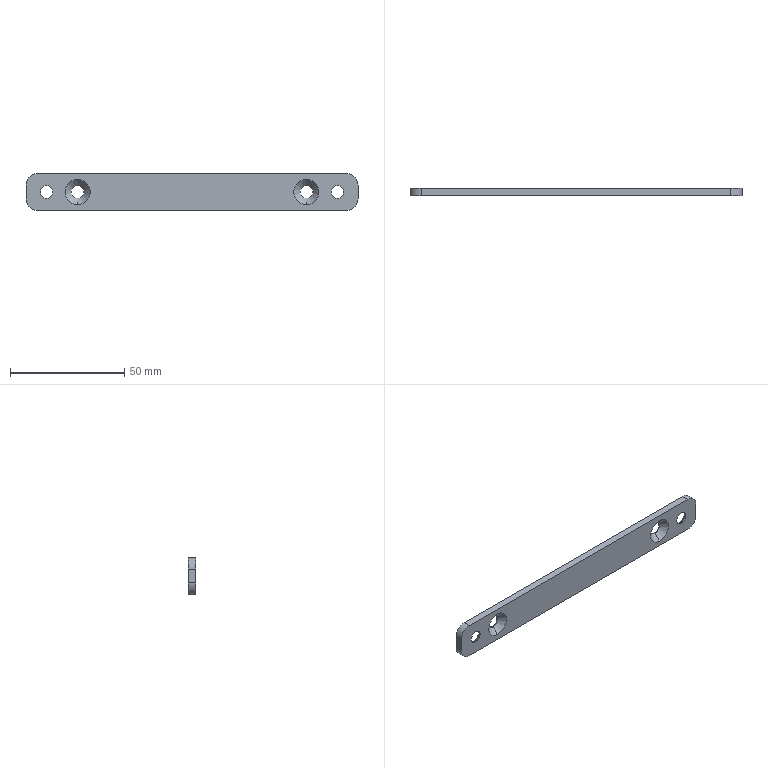Part | SolidWorks | features BaseBody 1 | 1 solid | 26 faces | box 145 x 3.2 x 16 mm | volume 6696 mm3 | cylinder 12 | cone 8 | plane 6 | commonest cylinder face diameters 5.5 x8 10 x4
STEP:
#1=CARTESIAN_POINT('',(0.,-0.4,2.75));
#2=VERTEX_POINT('',#1);
#3=CARTESIAN_POINT('',(0.,-0.4,-2.75));
#4=VERTEX_POINT('',#3);
#5=CARTESIAN_POINT('',(0.,-0.4,0.));
#6=DIRECTION('',(0.,-1.,0.));
#7=DIRECTION('',(1.,0.,0.));
#8=AXIS2_PLACEMENT_3D('',#5,#6,#7);
#9=CIRCLE('',#8,2.75);
#10=EDGE_CURVE('',#2,#4,#9,.T.);
#11=ORIENTED_EDGE('',*,*,#10,.F.);
#12=CARTESIAN_POINT('',(0.,-3.2,5.5));
#13=VERTEX_POINT('',#12);
#14=CARTESIAN_POINT('',(0.,-3.2,5.5));
#15=DIRECTION('',(0.,-0.7134,0.7007));
#16=VECTOR('',#15,1000.);
#17=LINE('',#14,#16);
#18=EDGE_CURVE('',#2,#13,#17,.T.);
#19=ORIENTED_EDGE('',*,*,#18,.T.);
#20=CARTESIAN_POINT('',(0.,-3.2,-5.5));
#21=VERTEX_POINT('',#20);
#22=CARTESIAN_POINT('',(0.,-3.2,0.));
#23=DIRECTION('',(0.,-1.,0.));
#24=DIRECTION('',(0.,0.,-1.));
#25=AXIS2_PLACEMENT_3D('',#22,#23,#24);
#26=CIRCLE('',#25,5.5);
#27=EDGE_CURVE('',#13,#21,#26,.T.);
#28=ORIENTED_EDGE('',*,*,#27,.T.);
#29=CARTESIAN_POINT('',(0.,-3.2,-5.5));
#30=DIRECTION('',(0.,-0.7134,-0.7007));
#31=VECTOR('',#30,1000.);
#32=LINE('',#29,#31);
#33=EDGE_CURVE('',#4,#21,#32,.T.);
#34=ORIENTED_EDGE('',*,*,#33,.F.);
#35=EDGE_LOOP('',(#11,#19,#28,#34));
#36=FACE_OUTER_BOUND('',#35,.T.);
#37=CARTESIAN_POINT('',(0.,-3.2,0.));
#38=DIRECTION('',(0.,-1.,0.));
#39=DIRECTION('',(0.,0.,-1.));
#40=AXIS2_PLACEMENT_3D('',#37,#38,#39);
#41=CONICAL_SURFACE('',#40,5.5,0.7764);
#42=ADVANCED_FACE('',(#36),#41,.F.);
#43=CARTESIAN_POINT('',(100.,-0.4,2.75));
#44=VERTEX_POINT('',#43);
#45=CARTESIAN_POINT('',(100.,-0.4,-2.75));
#46=VERTEX_POINT('',#45);
#47=CARTESIAN_POINT('',(100.,-0.4,0.));
#48=DIRECTION('',(0.,-1.,0.));
#49=DIRECTION('',(1.,0.,0.));
#50=AXIS2_PLACEMENT_3D('',#47,#48,#49);
#51=CIRCLE('',#50,2.75);
#52=EDGE_CURVE('',#44,#46,#51,.T.);
#53=ORIENTED_EDGE('',*,*,#52,.F.);
#54=CARTESIAN_POINT('',(100.,-3.2,5.5));
#55=VERTEX_POINT('',#54);
#56=CARTESIAN_POINT('',(100.,-3.2,5.5));
#57=DIRECTION('',(0.,-0.7134,0.7007));
#58=VECTOR('',#57,1000.);
#59=LINE('',#56,#58);
#60=EDGE_CURVE('',#44,#55,#59,.T.);
#61=ORIENTED_EDGE('',*,*,#60,.T.);
#62=CARTESIAN_POINT('',(100.,-3.2,-5.5));
#63=VERTEX_POINT('',#62);
#64=CARTESIAN_POINT('',(100.,-3.2,0.));
#65=DIRECTION('',(0.,-1.,0.));
#66=DIRECTION('',(0.,0.,-1.));
#67=AXIS2_PLACEMENT_3D('',#64,#65,#66);
#68=CIRCLE('',#67,5.5);
#69=EDGE_CURVE('',#55,#63,#68,.T.);
#70=ORIENTED_EDGE('',*,*,#69,.T.);
#71=CARTESIAN_POINT('',(100.,-3.2,-5.5));
#72=DIRECTION('',(0.,-0.7134,-0.7007));
#73=VECTOR('',#72,1000.);
#74=LINE('',#71,#73);
#75=EDGE_CURVE('',#46,#63,#74,.T.);
#76=ORIENTED_EDGE('',*,*,#75,.F.);
#77=EDGE_LOOP('',(#53,#61,#70,#76));
#78=FACE_OUTER_BOUND('',#77,.T.);
#79=CARTESIAN_POINT('',(100.,-3.2,0.));
#80=DIRECTION('',(0.,-1.,0.));
#81=DIRECTION('',(0.,0.,-1.));
#82=AXIS2_PLACEMENT_3D('',#79,#80,#81);
#83=CONICAL_SURFACE('',#82,5.5,0.7764);
#84=ADVANCED_FACE('',(#78),#83,.F.);
#85=CARTESIAN_POINT('',(-13.5,-3.2,2.75));
#86=VERTEX_POINT('',#85);
#87=CARTESIAN_POINT('',(-13.5,-3.2,-2.75));
#88=VERTEX_POINT('',#87);
#89=CARTESIAN_POINT('',(-13.5,-3.2,0.));
#90=DIRECTION('',(0.,-1.,0.));
#91=DIRECTION('',(0.,0.,1.));
#92=AXIS2_PLACEMENT_3D('',#89,#90,#91);
#93=CIRCLE('',#92,2.75);
#94=EDGE_CURVE('',#86,#88,#93,.T.);
#95=ORIENTED_EDGE('',*,*,#94,.T.);
#96=CARTESIAN_POINT('',(-13.5,-2.8,-2.75));
#97=VERTEX_POINT('',#96);
#98=CARTESIAN_POINT('',(-13.5,-3.,-2.75));
#99=DIRECTION('',(0.,1.,0.));
#100=VECTOR('',#99,1000.);
#101=LINE('',#98,#100);
#102=EDGE_CURVE('',#88,#97,#101,.T.);
#103=ORIENTED_EDGE('',*,*,#102,.T.);
#104=CARTESIAN_POINT('',(-13.5,-2.8,2.75));
#105=VERTEX_POINT('',#104);
#106=CARTESIAN_POINT('',(-13.5,-2.8,0.));
#107=DIRECTION('',(0.,-1.,0.));
#108=DIRECTION('',(0.,0.,1.));
#109=AXIS2_PLACEMENT_3D('',#106,#107,#108);
#110=CIRCLE('',#109,2.75);
#111=EDGE_CURVE('',#105,#97,#110,.T.);
#112=ORIENTED_EDGE('',*,*,#111,.F.);
#113=CARTESIAN_POINT('',(-13.5,-3.,2.75));
#114=DIRECTION('',(0.,1.,0.));
#115=VECTOR('',#114,1000.);
#116=LINE('',#113,#115);
#117=EDGE_CURVE('',#86,#105,#116,.T.);
#118=ORIENTED_EDGE('',*,*,#117,.F.);
#119=EDGE_LOOP('',(#95,#103,#112,#118));
#120=FACE_OUTER_BOUND('',#119,.T.);
#121=CARTESIAN_POINT('',(-13.5,-3.,0.));
#122=DIRECTION('',(0.,1.,0.));
#123=DIRECTION('',(0.,0.,1.));
#124=AXIS2_PLACEMENT_3D('',#121,#122,#123);
#125=CYLINDRICAL_SURFACE('',#124,2.75);
#126=ADVANCED_FACE('',(#120),#125,.F.);
#127=CARTESIAN_POINT('',(113.5,-3.2,2.75));
#128=VERTEX_POINT('',#127);
#129=CARTESIAN_POINT('',(113.5,-3.2,-2.75));
#130=VERTEX_POINT('',#129);
#131=CARTESIAN_POINT('',(113.5,-3.2,0.));
#132=DIRECTION('',(0.,-1.,0.));
#133=DIRECTION('',(0.,0.,1.));
#134=AXIS2_PLACEMENT_3D('',#131,#132,#133);
#135=CIRCLE('',#134,2.75);
#136=EDGE_CURVE('',#128,#130,#135,.T.);
#137=ORIENTED_EDGE('',*,*,#136,.T.);
#138=CARTESIAN_POINT('',(113.5,-2.8,-2.75));
#139=VERTEX_POINT('',#138);
#140=CARTESIAN_POINT('',(113.5,-3.,-2.75));
#141=DIRECTION('',(0.,1.,0.));
#142=VECTOR('',#141,1000.);
#143=LINE('',#140,#142);
#144=EDGE_CURVE('',#130,#139,#143,.T.);
#145=ORIENTED_EDGE('',*,*,#144,.T.);
#146=CARTESIAN_POINT('',(113.5,-2.8,2.75));
#147=VERTEX_POINT('',#146);
#148=CARTESIAN_POINT('',(113.5,-2.8,0.));
#149=DIRECTION('',(0.,-1.,0.));
#150=DIRECTION('',(0.,0.,1.));
#151=AXIS2_PLACEMENT_3D('',#148,#149,#150);
#152=CIRCLE('',#151,2.75);
#153=EDGE_CURVE('',#147,#139,#152,.T.);
#154=ORIENTED_EDGE('',*,*,#153,.F.);
#155=CARTESIAN_POINT('',(113.5,-3.,2.75));
#156=DIRECTION('',(0.,1.,0.));
#157=VECTOR('',#156,1000.);
#158=LINE('',#155,#157);
#159=EDGE_CURVE('',#128,#147,#158,.T.);
#160=ORIENTED_EDGE('',*,*,#159,.F.);
#161=EDGE_LOOP('',(#137,#145,#154,#160));
#162=FACE_OUTER_BOUND('',#161,.T.);
#163=CARTESIAN_POINT('',(113.5,-3.,0.));
#164=DIRECTION('',(0.,1.,0.));
#165=DIRECTION('',(0.,0.,1.));
#166=AXIS2_PLACEMENT_3D('',#163,#164,#165);
#167=CYLINDRICAL_SURFACE('',#166,2.75);
#168=ADVANCED_FACE('',(#162),#167,.F.);
#169=ORIENTED_EDGE('',*,*,#10,.T.);
#170=CARTESIAN_POINT('',(0.,0.,-2.75));
#171=VERTEX_POINT('',#170);
#172=CARTESIAN_POINT('',(0.,-0.2,-2.75));
#173=DIRECTION('',(0.,1.,0.));
#174=VECTOR('',#173,1000.);
#175=LINE('',#172,#174);
#176=EDGE_CURVE('',#4,#171,#175,.T.);
#177=ORIENTED_EDGE('',*,*,#176,.T.);
#178=CARTESIAN_POINT('',(0.,0.,2.75));
#179=VERTEX_POINT('',#178);
#180=CARTESIAN_POINT('',(0.,0.,0.));
#181=DIRECTION('',(0.,-1.,0.));
#182=DIRECTION('',(0.,0.,1.));
#183=AXIS2_PLACEMENT_3D('',#180,#181,#182);
#184=CIRCLE('',#183,2.75);
#185=EDGE_CURVE('',#179,#171,#184,.T.);
#186=ORIENTED_EDGE('',*,*,#185,.F.);
#187=CARTESIAN_POINT('',(0.,-0.2,2.75));
#188=DIRECTION('',(0.,1.,0.));
#189=VECTOR('',#188,1000.);
#190=LINE('',#187,#189);
#191=EDGE_CURVE('',#2,#179,#190,.T.);
#192=ORIENTED_EDGE('',*,*,#191,.F.);
#193=EDGE_LOOP('',(#169,#177,#186,#192));
#194=FACE_OUTER_BOUND('',#193,.T.);
#195=CARTESIAN_POINT('',(0.,-0.2,0.));
#196=DIRECTION('',(0.,1.,0.));
#197=DIRECTION('',(0.,0.,1.));
#198=AXIS2_PLACEMENT_3D('',#195,#196,#197);
#199=CYLINDRICAL_SURFACE('',#198,2.75);
#200=ADVANCED_FACE('',(#194),#199,.F.);
#201=ORIENTED_EDGE('',*,*,#52,.T.);
#202=CARTESIAN_POINT('',(100.,0.,-2.75));
#203=VERTEX_POINT('',#202);
#204=CARTESIAN_POINT('',(100.,-0.2,-2.75));
#205=DIRECTION('',(0.,1.,0.));
#206=VECTOR('',#205,1000.);
#207=LINE('',#204,#206);
#208=EDGE_CURVE('',#46,#203,#207,.T.);
#209=ORIENTED_EDGE('',*,*,#208,.T.);
#210=CARTESIAN_POINT('',(100.,0.,2.75));
#211=VERTEX_POINT('',#210);
#212=CARTESIAN_POINT('',(100.,0.,0.));
#213=DIRECTION('',(0.,-1.,0.));
#214=DIRECTION('',(0.,0.,1.));
#215=AXIS2_PLACEMENT_3D('',#212,#213,#214);
#216=CIRCLE('',#215,2.75);
#217=EDGE_CURVE('',#211,#203,#216,.T.);
#218=ORIENTED_EDGE('',*,*,#217,.F.);
#219=CARTESIAN_POINT('',(100.,-0.2,2.75));
#220=DIRECTION('',(0.,1.,0.));
#221=VECTOR('',#220,1000.);
#222=LINE('',#219,#221);
#223=EDGE_CURVE('',#44,#211,#222,.T.);
#224=ORIENTED_EDGE('',*,*,#223,.F.);
#225=EDGE_LOOP('',(#201,#209,#218,#224));
#226=FACE_OUTER_BOUND('',#225,.T.);
#227=CARTESIAN_POINT('',(100.,-0.2,0.));
#228=DIRECTION('',(0.,1.,0.));
#229=DIRECTION('',(0.,0.,1.));
#230=AXIS2_PLACEMENT_3D('',#227,#228,#229);
#231=CYLINDRICAL_SURFACE('',#230,2.75);
#232=ADVANCED_FACE('',(#226),#231,.F.);
#233=ORIENTED_EDGE('',*,*,#111,.T.);
#234=CARTESIAN_POINT('',(-13.5,0.,-5.5));
#235=VERTEX_POINT('',#234);
#236=CARTESIAN_POINT('',(-13.5,0.,-5.5));
#237=DIRECTION('',(0.,0.7134,-0.7007));
#238=VECTOR('',#237,1000.);
#239=LINE('',#236,#238);
#240=EDGE_CURVE('',#97,#235,#239,.T.);
#241=ORIENTED_EDGE('',*,*,#240,.T.);
#242=CARTESIAN_POINT('',(-13.5,0.,5.5));
#243=VERTEX_POINT('',#242);
#244=CARTESIAN_POINT('',(-13.5,0.,0.));
#245=DIRECTION('',(0.,-1.,0.));
#246=DIRECTION('',(0.,0.,1.));
#247=AXIS2_PLACEMENT_3D('',#244,#245,#246);
#248=CIRCLE('',#247,5.5);
#249=EDGE_CURVE('',#243,#235,#248,.T.);
#250=ORIENTED_EDGE('',*,*,#249,.F.);
#251=CARTESIAN_POINT('',(-13.5,0.,5.5));
#252=DIRECTION('',(0.,0.7134,0.7007));
#253=VECTOR('',#252,1000.);
#254=LINE('',#251,#253);
#255=EDGE_CURVE('',#105,#243,#254,.T.);
#256=ORIENTED_EDGE('',*,*,#255,.F.);
#257=EDGE_LOOP('',(#233,#241,#250,#256));
#258=FACE_OUTER_BOUND('',#257,.T.);
#259=CARTESIAN_POINT('',(-13.5,0.,0.));
#260=DIRECTION('',(0.,1.,0.));
#261=DIRECTION('',(0.,0.,1.));
#262=AXIS2_PLACEMENT_3D('',#259,#260,#261);
#263=CONICAL_SURFACE('',#262,5.5,0.7764);
#264=ADVANCED_FACE('',(#258),#263,.F.);
#265=ORIENTED_EDGE('',*,*,#153,.T.);
#266=CARTESIAN_POINT('',(113.5,0.,-5.5));
#267=VERTEX_POINT('',#266);
#268=CARTESIAN_POINT('',(113.5,0.,-5.5));
#269=DIRECTION('',(0.,0.7134,-0.7007));
#270=VECTOR('',#269,1000.);
#271=LINE('',#268,#270);
#272=EDGE_CURVE('',#139,#267,#271,.T.);
#273=ORIENTED_EDGE('',*,*,#272,.T.);
#274=CARTESIAN_POINT('',(113.5,0.,5.5));
#275=VERTEX_POINT('',#274);
#276=CARTESIAN_POINT('',(113.5,0.,0.));
#277=DIRECTION('',(0.,-1.,0.));
#278=DIRECTION('',(0.,0.,1.));
#279=AXIS2_PLACEMENT_3D('',#276,#277,#278);
#280=CIRCLE('',#279,5.5);
#281=EDGE_CURVE('',#275,#267,#280,.T.);
#282=ORIENTED_EDGE('',*,*,#281,.F.);
#283=CARTESIAN_POINT('',(113.5,0.,5.5));
#284=DIRECTION('',(0.,0.7134,0.7007));
#285=VECTOR('',#284,1000.);
#286=LINE('',#283,#285);
#287=EDGE_CURVE('',#147,#275,#286,.T.);
#288=ORIENTED_EDGE('',*,*,#287,.F.);
#289=EDGE_LOOP('',(#265,#273,#282,#288));
#290=FACE_OUTER_BOUND('',#289,.T.);
#291=CARTESIAN_POINT('',(113.5,0.,0.));
#292=DIRECTION('',(0.,1.,0.));
#293=DIRECTION('',(0.,0.,1.));
#294=AXIS2_PLACEMENT_3D('',#291,#292,#293);
#295=CONICAL_SURFACE('',#294,5.5,0.7764);
#296=ADVANCED_FACE('',(#290),#295,.F.);
#297=ORIENTED_EDGE('',*,*,#281,.T.);
#298=CARTESIAN_POINT('',(113.5,0.,0.));
#299=DIRECTION('',(0.,-1.,0.));
#300=DIRECTION('',(0.,0.,1.));
#301=AXIS2_PLACEMENT_3D('',#298,#299,#300);
#302=CIRCLE('',#301,5.5);
#303=EDGE_CURVE('',#267,#275,#302,.T.);
#304=ORIENTED_EDGE('',*,*,#303,.T.);
#305=EDGE_LOOP('',(#297,#304));
#306=FACE_BOUND('',#305,.T.);
#307=ORIENTED_EDGE('',*,*,#249,.T.);
#308=CARTESIAN_POINT('',(-13.5,0.,0.));
#309=DIRECTION('',(0.,-1.,0.));
#310=DIRECTION('',(0.,0.,1.));
#311=AXIS2_PLACEMENT_3D('',#308,#309,#310);
#312=CIRCLE('',#311,5.5);
#313=EDGE_CURVE('',#235,#243,#312,.T.);
#314=ORIENTED_EDGE('',*,*,#313,.T.);
#315=EDGE_LOOP('',(#307,#314));
#316=FACE_BOUND('',#315,.T.);
#317=ORIENTED_EDGE('',*,*,#217,.T.);
#318=CARTESIAN_POINT('',(100.,0.,0.));
#319=DIRECTION('',(0.,-1.,0.));
#320=DIRECTION('',(0.,0.,1.));
#321=AXIS2_PLACEMENT_3D('',#318,#319,#320);
#322=CIRCLE('',#321,2.75);
#323=EDGE_CURVE('',#203,#211,#322,.T.);
#324=ORIENTED_EDGE('',*,*,#323,.T.);
#325=EDGE_LOOP('',(#317,#324));
#326=FACE_BOUND('',#325,.T.);
#327=ORIENTED_EDGE('',*,*,#185,.T.);
#328=CARTESIAN_POINT('',(0.,0.,0.));
#329=DIRECTION('',(0.,-1.,0.));
#330=DIRECTION('',(0.,0.,1.));
#331=AXIS2_PLACEMENT_3D('',#328,#329,#330);
#332=CIRCLE('',#331,2.75);
#333=EDGE_CURVE('',#171,#179,#332,.T.);
#334=ORIENTED_EDGE('',*,*,#333,.T.);
#335=EDGE_LOOP('',(#327,#334));
#336=FACE_BOUND('',#335,.T.);
#337=CARTESIAN_POINT('',(-17.5,0.,-8.));
#338=VERTEX_POINT('',#337);
#339=CARTESIAN_POINT('',(117.5,0.,-8.));
#340=VERTEX_POINT('',#339);
#341=CARTESIAN_POINT('',(117.5,0.,-8.));
#342=DIRECTION('',(1.,0.,0.));
#343=VECTOR('',#342,1000.);
#344=LINE('',#341,#343);
#345=EDGE_CURVE('',#338,#340,#344,.T.);
#346=ORIENTED_EDGE('',*,*,#345,.F.);
#347=CARTESIAN_POINT('',(-22.5,0.,-3.));
#348=VERTEX_POINT('',#347);
#349=CARTESIAN_POINT('',(-17.5,0.,-3.));
#350=DIRECTION('',(0.,-1.,0.));
#351=DIRECTION('',(0.,0.,1.));
#352=AXIS2_PLACEMENT_3D('',#349,#350,#351);
#353=CIRCLE('',#352,5.);
#354=EDGE_CURVE('',#348,#338,#353,.T.);
#355=ORIENTED_EDGE('',*,*,#354,.F.);
#356=CARTESIAN_POINT('',(-22.5,0.,3.));
#357=VERTEX_POINT('',#356);
#358=CARTESIAN_POINT('',(-22.5,0.,-3.));
#359=DIRECTION('',(0.,0.,-1.));
#360=VECTOR('',#359,1000.);
#361=LINE('',#358,#360);
#362=EDGE_CURVE('',#357,#348,#361,.T.);
#363=ORIENTED_EDGE('',*,*,#362,.F.);
#364=CARTESIAN_POINT('',(-17.5,0.,8.));
#365=VERTEX_POINT('',#364);
#366=CARTESIAN_POINT('',(-17.5,0.,3.));
#367=DIRECTION('',(0.,-1.,0.));
#368=DIRECTION('',(0.,0.,1.));
#369=AXIS2_PLACEMENT_3D('',#366,#367,#368);
#370=CIRCLE('',#369,5.);
#371=EDGE_CURVE('',#365,#357,#370,.T.);
#372=ORIENTED_EDGE('',*,*,#371,.F.);
#373=CARTESIAN_POINT('',(117.5,0.,8.));
#374=VERTEX_POINT('',#373);
#375=CARTESIAN_POINT('',(-17.5,0.,8.));
#376=DIRECTION('',(-1.,0.,0.));
#377=VECTOR('',#376,1000.);
#378=LINE('',#375,#377);
#379=EDGE_CURVE('',#374,#365,#378,.T.);
#380=ORIENTED_EDGE('',*,*,#379,.F.);
#381=CARTESIAN_POINT('',(122.5,0.,3.));
#382=VERTEX_POINT('',#381);
#383=CARTESIAN_POINT('',(117.5,0.,3.));
#384=DIRECTION('',(0.,-1.,0.));
#385=DIRECTION('',(0.,0.,1.));
#386=AXIS2_PLACEMENT_3D('',#383,#384,#385);
#387=CIRCLE('',#386,5.);
#388=EDGE_CURVE('',#382,#374,#387,.T.);
#389=ORIENTED_EDGE('',*,*,#388,.F.);
#390=CARTESIAN_POINT('',(122.5,0.,-3.));
#391=VERTEX_POINT('',#390);
#392=CARTESIAN_POINT('',(122.5,0.,3.));
#393=DIRECTION('',(0.,0.,1.));
#394=VECTOR('',#393,1000.);
#395=LINE('',#392,#394);
#396=EDGE_CURVE('',#391,#382,#395,.T.);
#397=ORIENTED_EDGE('',*,*,#396,.F.);
#398=CARTESIAN_POINT('',(117.5,0.,-3.));
#399=DIRECTION('',(0.,-1.,0.));
#400=DIRECTION('',(0.,0.,1.));
#401=AXIS2_PLACEMENT_3D('',#398,#399,#400);
#402=CIRCLE('',#401,5.);
#403=EDGE_CURVE('',#340,#391,#402,.T.);
#404=ORIENTED_EDGE('',*,*,#403,.F.);
#405=EDGE_LOOP('',(#346,#355,#363,#372,#380,#389,#397,#404));
#406=FACE_OUTER_BOUND('',#405,.T.);
#407=CARTESIAN_POINT('',(50.,0.,0.));
#408=DIRECTION('',(0.,1.,0.));
#409=DIRECTION('',(1.,0.,0.));
#410=AXIS2_PLACEMENT_3D('',#407,#408,#409);
#411=PLANE('',#410);
#412=ADVANCED_FACE('',(#306,#316,#326,#336,#406),#411,.T.);
#413=ORIENTED_EDGE('',*,*,#379,.T.);
#414=CARTESIAN_POINT('',(-17.5,-3.2,8.));
#415=VERTEX_POINT('',#414);
#416=CARTESIAN_POINT('',(-17.5,0.,8.));
#417=DIRECTION('',(0.,1.,0.));
#418=VECTOR('',#417,1000.);
#419=LINE('',#416,#418);
#420=EDGE_CURVE('',#415,#365,#419,.T.);
#421=ORIENTED_EDGE('',*,*,#420,.F.);
#422=CARTESIAN_POINT('',(117.5,-3.2,8.));
#423=VERTEX_POINT('',#422);
#424=CARTESIAN_POINT('',(50.,-3.2,8.));
#425=DIRECTION('',(1.,0.,0.));
#426=VECTOR('',#425,1000.);
#427=LINE('',#424,#426);
#428=EDGE_CURVE('',#415,#423,#427,.T.);
#429=ORIENTED_EDGE('',*,*,#428,.T.);
#430=CARTESIAN_POINT('',(117.5,0.,8.));
#431=DIRECTION('',(0.,-1.,0.));
#432=VECTOR('',#431,1000.);
#433=LINE('',#430,#432);
#434=EDGE_CURVE('',#374,#423,#433,.T.);
#435=ORIENTED_EDGE('',*,*,#434,.F.);
#436=EDGE_LOOP('',(#413,#421,#429,#435));
#437=FACE_OUTER_BOUND('',#436,.T.);
#438=CARTESIAN_POINT('',(-17.5,0.,8.));
#439=DIRECTION('',(0.,0.,1.));
#440=DIRECTION('',(1.,0.,0.));
#441=AXIS2_PLACEMENT_3D('',#438,#439,#440);
#442=PLANE('',#441);
#443=ADVANCED_FACE('',(#437),#442,.T.);
#444=ORIENTED_EDGE('',*,*,#388,.T.);
#445=ORIENTED_EDGE('',*,*,#434,.T.);
#446=CARTESIAN_POINT('',(122.5,-3.2,3.));
#447=VERTEX_POINT('',#446);
#448=CARTESIAN_POINT('',(117.5,-3.2,3.));
#449=DIRECTION('',(0.,1.,0.));
#450=DIRECTION('',(0.,0.,1.));
#451=AXIS2_PLACEMENT_3D('',#448,#449,#450);
#452=CIRCLE('',#451,5.);
#453=EDGE_CURVE('',#423,#447,#452,.T.);
#454=ORIENTED_EDGE('',*,*,#453,.T.);
#455=CARTESIAN_POINT('',(122.5,0.,3.));
#456=DIRECTION('',(0.,-1.,0.));
#457=VECTOR('',#456,1000.);
#458=LINE('',#455,#457);
#459=EDGE_CURVE('',#382,#447,#458,.T.);
#460=ORIENTED_EDGE('',*,*,#459,.F.);
#461=EDGE_LOOP('',(#444,#445,#454,#460));
#462=FACE_OUTER_BOUND('',#461,.T.);
#463=CARTESIAN_POINT('',(117.5,0.,3.));
#464=DIRECTION('',(0.,1.,0.));
#465=DIRECTION('',(0.,0.,1.));
#466=AXIS2_PLACEMENT_3D('',#463,#464,#465);
#467=CYLINDRICAL_SURFACE('',#466,5.);
#468=ADVANCED_FACE('',(#462),#467,.T.);
#469=ORIENTED_EDGE('',*,*,#396,.T.);
#470=ORIENTED_EDGE('',*,*,#459,.T.);
#471=CARTESIAN_POINT('',(122.5,-3.2,-3.));
#472=VERTEX_POINT('',#471);
#473=CARTESIAN_POINT('',(122.5,-3.2,0.));
#474=DIRECTION('',(0.,0.,-1.));
#475=VECTOR('',#474,1000.);
#476=LINE('',#473,#475);
#477=EDGE_CURVE('',#447,#472,#476,.T.);
#478=ORIENTED_EDGE('',*,*,#477,.T.);
#479=CARTESIAN_POINT('',(122.5,0.,-3.));
#480=DIRECTION('',(0.,-1.,0.));
#481=VECTOR('',#480,1000.);
#482=LINE('',#479,#481);
#483=EDGE_CURVE('',#391,#472,#482,.T.);
#484=ORIENTED_EDGE('',*,*,#483,.F.);
#485=EDGE_LOOP('',(#469,#470,#478,#484));
#486=FACE_OUTER_BOUND('',#485,.T.);
#487=CARTESIAN_POINT('',(122.5,0.,3.));
#488=DIRECTION('',(1.,0.,0.));
#489=DIRECTION('',(0.,1.,0.));
#490=AXIS2_PLACEMENT_3D('',#487,#488,#489);
#491=PLANE('',#490);
#492=ADVANCED_FACE('',(#486),#491,.T.);
#493=ORIENTED_EDGE('',*,*,#403,.T.);
#494=ORIENTED_EDGE('',*,*,#483,.T.);
#495=CARTESIAN_POINT('',(117.5,-3.2,-8.));
#496=VERTEX_POINT('',#495);
#497=CARTESIAN_POINT('',(117.5,-3.2,-3.));
#498=DIRECTION('',(0.,1.,0.));
#499=DIRECTION('',(0.,0.,1.));
#500=AXIS2_PLACEMENT_3D('',#497,#498,#499);
#501=CIRCLE('',#500,5.);
#502=EDGE_CURVE('',#472,#496,#501,.T.);
#503=ORIENTED_EDGE('',*,*,#502,.T.);
#504=CARTESIAN_POINT('',(117.5,0.,-8.));
#505=DIRECTION('',(0.,-1.,0.));
#506=VECTOR('',#505,1000.);
#507=LINE('',#504,#506);
#508=EDGE_CURVE('',#340,#496,#507,.T.);
#509=ORIENTED_EDGE('',*,*,#508,.F.);
#510=EDGE_LOOP('',(#493,#494,#503,#509));
#511=FACE_OUTER_BOUND('',#510,.T.);
#512=CARTESIAN_POINT('',(117.5,0.,-3.));
#513=DIRECTION('',(0.,1.,0.));
#514=DIRECTION('',(0.,0.,1.));
#515=AXIS2_PLACEMENT_3D('',#512,#513,#514);
#516=CYLINDRICAL_SURFACE('',#515,5.);
#517=ADVANCED_FACE('',(#511),#516,.T.);
#518=ORIENTED_EDGE('',*,*,#345,.T.);
#519=ORIENTED_EDGE('',*,*,#508,.T.);
#520=CARTESIAN_POINT('',(-17.5,-3.2,-8.));
#521=VERTEX_POINT('',#520);
#522=CARTESIAN_POINT('',(50.,-3.2,-8.));
#523=DIRECTION('',(-1.,0.,0.));
#524=VECTOR('',#523,1000.);
#525=LINE('',#522,#524);
#526=EDGE_CURVE('',#496,#521,#525,.T.);
#527=ORIENTED_EDGE('',*,*,#526,.T.);
#528=CARTESIAN_POINT('',(-17.5,0.,-8.));
#529=DIRECTION('',(0.,-1.,0.));
#530=VECTOR('',#529,1000.);
#531=LINE('',#528,#530);
#532=EDGE_CURVE('',#338,#521,#531,.T.);
#533=ORIENTED_EDGE('',*,*,#532,.F.);
#534=EDGE_LOOP('',(#518,#519,#527,#533));
#535=FACE_OUTER_BOUND('',#534,.T.);
#536=CARTESIAN_POINT('',(117.5,0.,-8.));
#537=DIRECTION('',(0.,0.,-1.));
#538=DIRECTION('',(0.,-1.,0.));
#539=AXIS2_PLACEMENT_3D('',#536,#537,#538);
#540=PLANE('',#539);
#541=ADVANCED_FACE('',(#535),#540,.T.);
#542=ORIENTED_EDGE('',*,*,#354,.T.);
#543=ORIENTED_EDGE('',*,*,#532,.T.);
#544=CARTESIAN_POINT('',(-22.5,-3.2,-3.));
#545=VERTEX_POINT('',#544);
#546=CARTESIAN_POINT('',(-17.5,-3.2,-3.));
#547=DIRECTION('',(0.,1.,0.));
#548=DIRECTION('',(0.,0.,1.));
#549=AXIS2_PLACEMENT_3D('',#546,#547,#548);
#550=CIRCLE('',#549,5.);
#551=EDGE_CURVE('',#521,#545,#550,.T.);
#552=ORIENTED_EDGE('',*,*,#551,.T.);
#553=CARTESIAN_POINT('',(-22.5,0.,-3.));
#554=DIRECTION('',(0.,-1.,0.));
#555=VECTOR('',#554,1000.);
#556=LINE('',#553,#555);
#557=EDGE_CURVE('',#348,#545,#556,.T.);
#558=ORIENTED_EDGE('',*,*,#557,.F.);
#559=EDGE_LOOP('',(#542,#543,#552,#558));
#560=FACE_OUTER_BOUND('',#559,.T.);
#561=CARTESIAN_POINT('',(-17.5,0.,-3.));
#562=DIRECTION('',(0.,1.,0.));
#563=DIRECTION('',(0.,0.,1.));
#564=AXIS2_PLACEMENT_3D('',#561,#562,#563);
#565=CYLINDRICAL_SURFACE('',#564,5.);
#566=ADVANCED_FACE('',(#560),#565,.T.);
#567=ORIENTED_EDGE('',*,*,#362,.T.);
#568=ORIENTED_EDGE('',*,*,#557,.T.);
#569=CARTESIAN_POINT('',(-22.5,-3.2,3.));
#570=VERTEX_POINT('',#569);
#571=CARTESIAN_POINT('',(-22.5,-3.2,0.));
#572=DIRECTION('',(0.,0.,1.));
#573=VECTOR('',#572,1000.);
#574=LINE('',#571,#573);
#575=EDGE_CURVE('',#545,#570,#574,.T.);
#576=ORIENTED_EDGE('',*,*,#575,.T.);
#577=CARTESIAN_POINT('',(-22.5,0.,3.));
#578=DIRECTION('',(0.,-1.,0.));
#579=VECTOR('',#578,1000.);
#580=LINE('',#577,#579);
#581=EDGE_CURVE('',#357,#570,#580,.T.);
#582=ORIENTED_EDGE('',*,*,#581,.F.);
#583=EDGE_LOOP('',(#567,#568,#576,#582));
#584=FACE_OUTER_BOUND('',#583,.T.);
#585=CARTESIAN_POINT('',(-22.5,0.,-3.));
#586=DIRECTION('',(-1.,0.,0.));
#587=DIRECTION('',(0.,0.,1.));
#588=AXIS2_PLACEMENT_3D('',#585,#586,#587);
#589=PLANE('',#588);
#590=ADVANCED_FACE('',(#584),#589,.T.);
#591=ORIENTED_EDGE('',*,*,#371,.T.);
#592=ORIENTED_EDGE('',*,*,#581,.T.);
#593=CARTESIAN_POINT('',(-17.5,-3.2,3.));
#594=DIRECTION('',(0.,1.,0.));
#595=DIRECTION('',(0.,0.,1.));
#596=AXIS2_PLACEMENT_3D('',#593,#594,#595);
#597=CIRCLE('',#596,5.);
#598=EDGE_CURVE('',#570,#415,#597,.T.);
#599=ORIENTED_EDGE('',*,*,#598,.T.);
#600=ORIENTED_EDGE('',*,*,#420,.T.);
#601=EDGE_LOOP('',(#591,#592,#599,#600));
#602=FACE_OUTER_BOUND('',#601,.T.);
#603=CARTESIAN_POINT('',(-17.5,0.,3.));
#604=DIRECTION('',(0.,1.,0.));
#605=DIRECTION('',(0.,0.,1.));
#606=AXIS2_PLACEMENT_3D('',#603,#604,#605);
#607=CYLINDRICAL_SURFACE('',#606,5.);
#608=ADVANCED_FACE('',(#602),#607,.T.);
#609=ORIENTED_EDGE('',*,*,#136,.F.);
#610=CARTESIAN_POINT('',(113.5,-3.2,0.));
#611=DIRECTION('',(0.,-1.,0.));
#612=DIRECTION('',(0.,0.,1.));
#613=AXIS2_PLACEMENT_3D('',#610,#611,#612);
#614=CIRCLE('',#613,2.75);
#615=EDGE_CURVE('',#130,#128,#614,.T.);
#616=ORIENTED_EDGE('',*,*,#615,.F.);
#617=EDGE_LOOP('',(#609,#616));
#618=FACE_BOUND('',#617,.T.);
#619=ORIENTED_EDGE('',*,*,#94,.F.);
#620=CARTESIAN_POINT('',(-13.5,-3.2,0.));
#621=DIRECTION('',(0.,-1.,0.));
#622=DIRECTION('',(0.,0.,1.));
#623=AXIS2_PLACEMENT_3D('',#620,#621,#622);
#624=CIRCLE('',#623,2.75);
#625=EDGE_CURVE('',#88,#86,#624,.T.);
#626=ORIENTED_EDGE('',*,*,#625,.F.);
#627=EDGE_LOOP('',(#619,#626));
#628=FACE_BOUND('',#627,.T.);
#629=CARTESIAN_POINT('',(100.,-3.2,0.));
#630=DIRECTION('',(0.,-1.,0.));
#631=DIRECTION('',(0.,0.,-1.));
#632=AXIS2_PLACEMENT_3D('',#629,#630,#631);
#633=CIRCLE('',#632,5.5);
#634=EDGE_CURVE('',#63,#55,#633,.T.);
#635=ORIENTED_EDGE('',*,*,#634,.F.);
#636=ORIENTED_EDGE('',*,*,#69,.F.);
#637=EDGE_LOOP('',(#635,#636));
#638=FACE_BOUND('',#637,.T.);
#639=CARTESIAN_POINT('',(0.,-3.2,0.));
#640=DIRECTION('',(0.,-1.,0.));
#641=DIRECTION('',(0.,0.,-1.));
#642=AXIS2_PLACEMENT_3D('',#639,#640,#641);
#643=CIRCLE('',#642,5.5);
#644=EDGE_CURVE('',#21,#13,#643,.T.);
#645=ORIENTED_EDGE('',*,*,#644,.F.);
#646=ORIENTED_EDGE('',*,*,#27,.F.);
#647=EDGE_LOOP('',(#645,#646));
#648=FACE_BOUND('',#647,.T.);
#649=ORIENTED_EDGE('',*,*,#575,.F.);
#650=ORIENTED_EDGE('',*,*,#551,.F.);
#651=ORIENTED_EDGE('',*,*,#526,.F.);
#652=ORIENTED_EDGE('',*,*,#502,.F.);
#653=ORIENTED_EDGE('',*,*,#477,.F.);
#654=ORIENTED_EDGE('',*,*,#453,.F.);
#655=ORIENTED_EDGE('',*,*,#428,.F.);
#656=ORIENTED_EDGE('',*,*,#598,.F.);
#657=EDGE_LOOP('',(#649,#650,#651,#652,#653,#654,#655,#656));
#658=FACE_OUTER_BOUND('',#657,.T.);
#659=CARTESIAN_POINT('',(50.,-3.2,0.));
#660=DIRECTION('',(0.,1.,0.));
#661=DIRECTION('',(1.,0.,0.));
#662=AXIS2_PLACEMENT_3D('',#659,#660,#661);
#663=PLANE('',#662);
#664=ADVANCED_FACE('',(#618,#628,#638,#648,#658),#663,.F.);
#665=ORIENTED_EDGE('',*,*,#272,.F.);
#666=CARTESIAN_POINT('',(113.5,-2.8,0.));
#667=DIRECTION('',(0.,-1.,0.));
#668=DIRECTION('',(0.,0.,1.));
#669=AXIS2_PLACEMENT_3D('',#666,#667,#668);
#670=CIRCLE('',#669,2.75);
#671=EDGE_CURVE('',#139,#147,#670,.T.);
#672=ORIENTED_EDGE('',*,*,#671,.T.);
#673=ORIENTED_EDGE('',*,*,#287,.T.);
#674=ORIENTED_EDGE('',*,*,#303,.F.);
#675=EDGE_LOOP('',(#665,#672,#673,#674));
#676=FACE_OUTER_BOUND('',#675,.T.);
#677=CARTESIAN_POINT('',(113.5,0.,0.));
#678=DIRECTION('',(0.,1.,0.));
#679=DIRECTION('',(0.,0.,1.));
#680=AXIS2_PLACEMENT_3D('',#677,#678,#679);
#681=CONICAL_SURFACE('',#680,5.5,0.7764);
#682=ADVANCED_FACE('',(#676),#681,.F.);
#683=ORIENTED_EDGE('',*,*,#240,.F.);
#684=CARTESIAN_POINT('',(-13.5,-2.8,0.));
#685=DIRECTION('',(0.,-1.,0.));
#686=DIRECTION('',(0.,0.,1.));
#687=AXIS2_PLACEMENT_3D('',#684,#685,#686);
#688=CIRCLE('',#687,2.75);
#689=EDGE_CURVE('',#97,#105,#688,.T.);
#690=ORIENTED_EDGE('',*,*,#689,.T.);
#691=ORIENTED_EDGE('',*,*,#255,.T.);
#692=ORIENTED_EDGE('',*,*,#313,.F.);
#693=EDGE_LOOP('',(#683,#690,#691,#692));
#694=FACE_OUTER_BOUND('',#693,.T.);
#695=CARTESIAN_POINT('',(-13.5,0.,0.));
#696=DIRECTION('',(0.,1.,0.));
#697=DIRECTION('',(0.,0.,1.));
#698=AXIS2_PLACEMENT_3D('',#695,#696,#697);
#699=CONICAL_SURFACE('',#698,5.5,0.7764);
#700=ADVANCED_FACE('',(#694),#699,.F.);
#701=ORIENTED_EDGE('',*,*,#208,.F.);
#702=CARTESIAN_POINT('',(100.,-0.4,0.));
#703=DIRECTION('',(0.,-1.,0.));
#704=DIRECTION('',(1.,0.,0.));
#705=AXIS2_PLACEMENT_3D('',#702,#703,#704);
#706=CIRCLE('',#705,2.75);
#707=EDGE_CURVE('',#46,#44,#706,.T.);
#708=ORIENTED_EDGE('',*,*,#707,.T.);
#709=ORIENTED_EDGE('',*,*,#223,.T.);
#710=ORIENTED_EDGE('',*,*,#323,.F.);
#711=EDGE_LOOP('',(#701,#708,#709,#710));
#712=FACE_OUTER_BOUND('',#711,.T.);
#713=CARTESIAN_POINT('',(100.,-0.2,0.));
#714=DIRECTION('',(0.,1.,0.));
#715=DIRECTION('',(0.,0.,1.));
#716=AXIS2_PLACEMENT_3D('',#713,#714,#715);
#717=CYLINDRICAL_SURFACE('',#716,2.75);
#718=ADVANCED_FACE('',(#712),#717,.F.);
#719=ORIENTED_EDGE('',*,*,#176,.F.);
#720=CARTESIAN_POINT('',(0.,-0.4,0.));
#721=DIRECTION('',(0.,-1.,0.));
#722=DIRECTION('',(1.,0.,0.));
#723=AXIS2_PLACEMENT_3D('',#720,#721,#722);
#724=CIRCLE('',#723,2.75);
#725=EDGE_CURVE('',#4,#2,#724,.T.);
#726=ORIENTED_EDGE('',*,*,#725,.T.);
#727=ORIENTED_EDGE('',*,*,#191,.T.);
#728=ORIENTED_EDGE('',*,*,#333,.F.);
#729=EDGE_LOOP('',(#719,#726,#727,#728));
#730=FACE_OUTER_BOUND('',#729,.T.);
#731=CARTESIAN_POINT('',(0.,-0.2,0.));
#732=DIRECTION('',(0.,1.,0.));
#733=DIRECTION('',(0.,0.,1.));
#734=AXIS2_PLACEMENT_3D('',#731,#732,#733);
#735=CYLINDRICAL_SURFACE('',#734,2.75);
#736=ADVANCED_FACE('',(#730),#735,.F.);
#737=ORIENTED_EDGE('',*,*,#144,.F.);
#738=ORIENTED_EDGE('',*,*,#615,.T.);
#739=ORIENTED_EDGE('',*,*,#159,.T.);
#740=ORIENTED_EDGE('',*,*,#671,.F.);
#741=EDGE_LOOP('',(#737,#738,#739,#740));
#742=FACE_OUTER_BOUND('',#741,.T.);
#743=CARTESIAN_POINT('',(113.5,-3.,0.));
#744=DIRECTION('',(0.,1.,0.));
#745=DIRECTION('',(0.,0.,1.));
#746=AXIS2_PLACEMENT_3D('',#743,#744,#745);
#747=CYLINDRICAL_SURFACE('',#746,2.75);
#748=ADVANCED_FACE('',(#742),#747,.F.);
#749=ORIENTED_EDGE('',*,*,#102,.F.);
#750=ORIENTED_EDGE('',*,*,#625,.T.);
#751=ORIENTED_EDGE('',*,*,#117,.T.);
#752=ORIENTED_EDGE('',*,*,#689,.F.);
#753=EDGE_LOOP('',(#749,#750,#751,#752));
#754=FACE_OUTER_BOUND('',#753,.T.);
#755=CARTESIAN_POINT('',(-13.5,-3.,0.));
#756=DIRECTION('',(0.,1.,0.));
#757=DIRECTION('',(0.,0.,1.));
#758=AXIS2_PLACEMENT_3D('',#755,#756,#757);
#759=CYLINDRICAL_SURFACE('',#758,2.75);
#760=ADVANCED_FACE('',(#754),#759,.F.);
#761=ORIENTED_EDGE('',*,*,#60,.F.);
#762=ORIENTED_EDGE('',*,*,#707,.F.);
#763=ORIENTED_EDGE('',*,*,#75,.T.);
#764=ORIENTED_EDGE('',*,*,#634,.T.);
#765=EDGE_LOOP('',(#761,#762,#763,#764));
#766=FACE_OUTER_BOUND('',#765,.T.);
#767=CARTESIAN_POINT('',(100.,-3.2,0.));
#768=DIRECTION('',(0.,-1.,0.));
#769=DIRECTION('',(0.,0.,-1.));
#770=AXIS2_PLACEMENT_3D('',#767,#768,#769);
#771=CONICAL_SURFACE('',#770,5.5,0.7764);
#772=ADVANCED_FACE('',(#766),#771,.F.);
#773=ORIENTED_EDGE('',*,*,#18,.F.);
#774=ORIENTED_EDGE('',*,*,#725,.F.);
#775=ORIENTED_EDGE('',*,*,#33,.T.);
#776=ORIENTED_EDGE('',*,*,#644,.T.);
#777=EDGE_LOOP('',(#773,#774,#775,#776));
#778=FACE_OUTER_BOUND('',#777,.T.);
#779=CARTESIAN_POINT('',(0.,-3.2,0.));
#780=DIRECTION('',(0.,-1.,0.));
#781=DIRECTION('',(0.,0.,-1.));
#782=AXIS2_PLACEMENT_3D('',#779,#780,#781);
#783=CONICAL_SURFACE('',#782,5.5,0.7764);
#784=ADVANCED_FACE('',(#778),#783,.F.);
#785=CLOSED_SHELL('',(#42,#84,#126,#168,#200,#232,#264,#296,#412,#443,#468,#492,#517,#541,#566,#590,#608,#664,#682,#700,#718,#736,#748,#760,#772,#784));
#786=MANIFOLD_SOLID_BREP('',#785);
#787=CARTESIAN_POINT('',(0.,0.,0.));
#788=DIRECTION('',(0.,0.,1.));
#789=DIRECTION('',(1.,0.,0.));
#790=AXIS2_PLACEMENT_3D('',#787,#788,#789);
#791=(LENGTH_UNIT()NAMED_UNIT(*)SI_UNIT(.MILLI.,.METRE.));
#792=UNCERTAINTY_MEASURE_WITH_UNIT(LENGTH_MEASURE(0.00001),#791,'','');
#793=(NAMED_UNIT(*)PLANE_ANGLE_UNIT()SI_UNIT($,.RADIAN.));
#794=(NAMED_UNIT(*)SI_UNIT($,.STERADIAN.)SOLID_ANGLE_UNIT());
#795=(GEOMETRIC_REPRESENTATION_CONTEXT(3)GLOBAL_UNCERTAINTY_ASSIGNED_CONTEXT((#792))GLOBAL_UNIT_ASSIGNED_CONTEXT((#791,#793,#794))REPRESENTATION_CONTEXT('',''));
#796=ADVANCED_BREP_SHAPE_REPRESENTATION('',(#786,#790),#795);